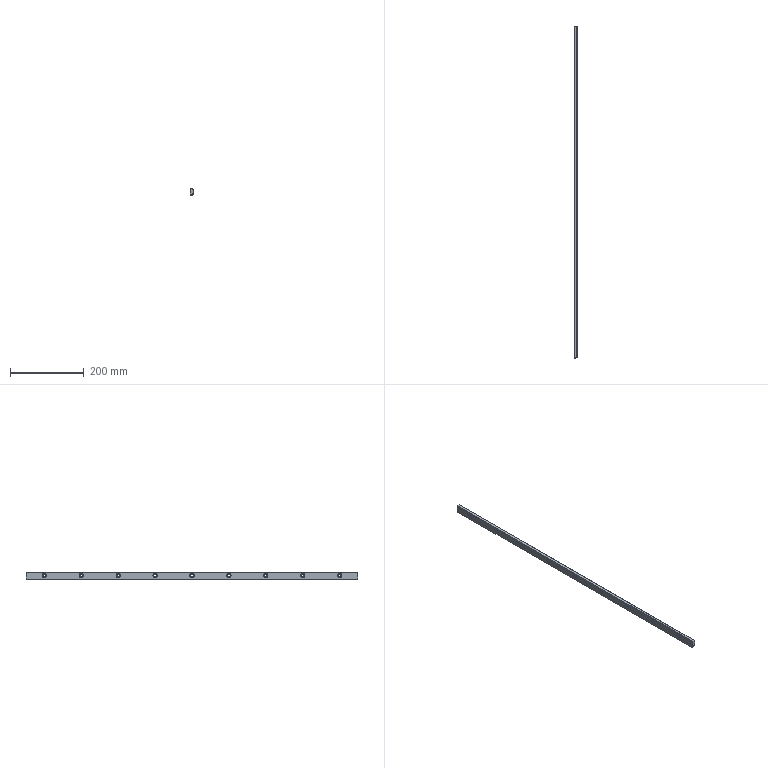Part | STEP file | 06B side guide-wheel chain support block | 1 solid | 63 faces | box 9 x 900 x 20.4 mm | volume 141982 mm3 | cylinder 42 | plane 21 | commonest cylinder face diameters 6.5 x18 12 x18 3 x6